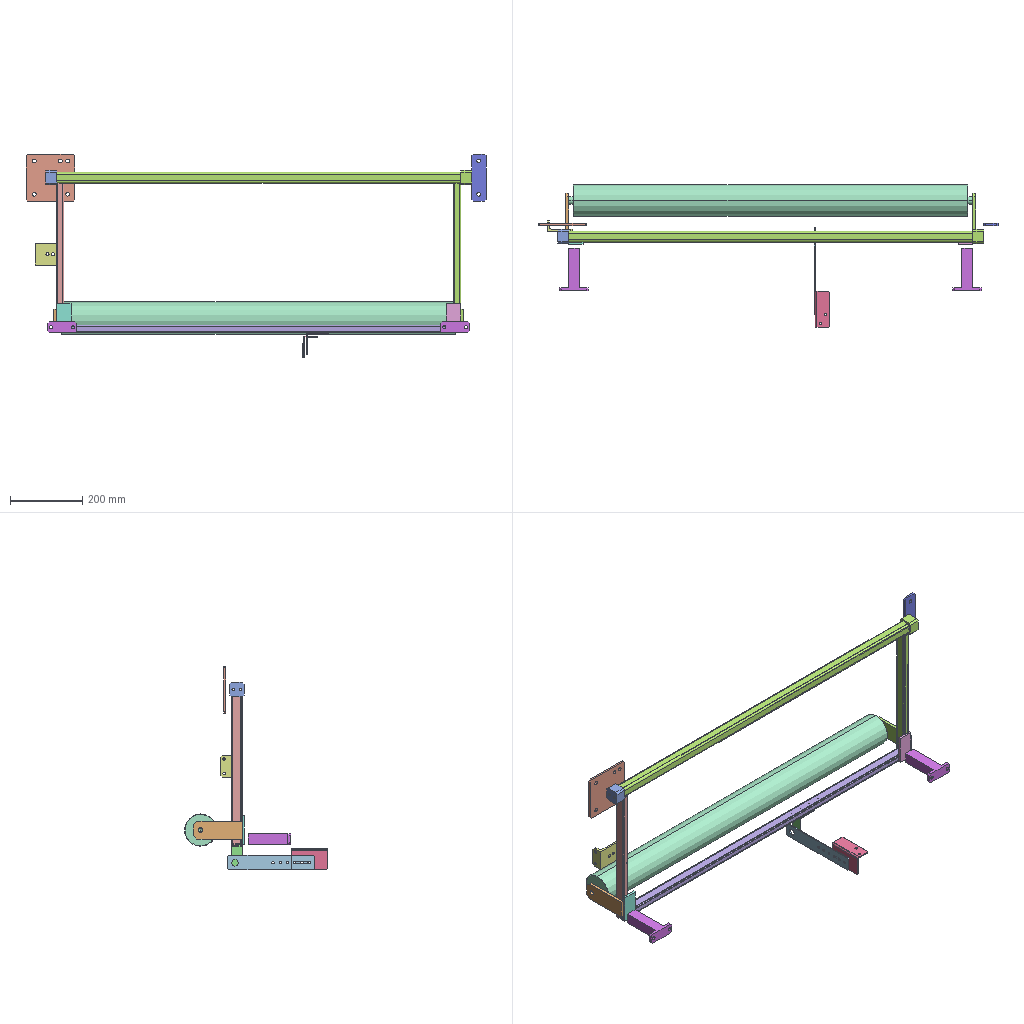Assembly | SolidWorks | 10 different items | 11 placed | box 1270 x 394 x 563 mm
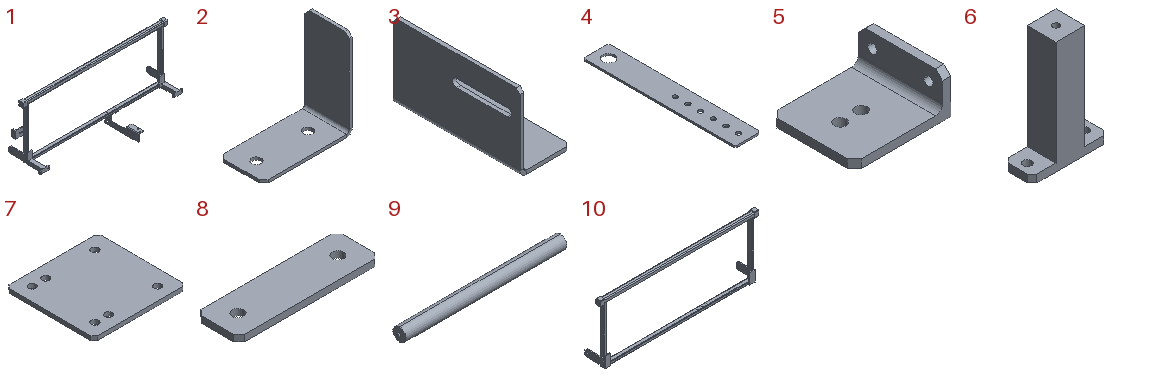Parts list (item | name | quantity | parent item | size | volume | features):
1 | (subassembly) | x1 | - | 1205 x 370 x 518 mm | 1223127 mm3 | -
2 | - | x1 | in 1 | 60 x 30 x 60 mm | 6834 mm3 | features Chamfer 1, EdgeFlange 1, FlatPattern 1, ICE 1, SMBaseFlange 1, SheetMetal 1
3 | - | x1 | in 1 | 40 x 100 x 60 mm | 27517 mm3 | features Chamfer 1, EdgeFlange 1, FlatPattern 1, ICE 1, SMBaseFlange 1, SheetMetal 1
4 | - | x1 | in 1 | 40 x 240 x 3 mm | 27247 mm3 | features Extrusion 1
5 | - | x1 | in 1 | 69 x 60 x 30 mm | 32423 mm3 | features ICE 3, Chamfer 1, Extrusion 1, Fillet 1
6 | - | x2 | in 1 | 80 x 30 x 118 mm | 115849 mm3 | features ICE 2, 3DProfileFeature 1, Extrusion 1, HoleWzd 1
7 | - | x1 | - | 135 x 130 x 6 mm | 101883 mm3 | features Extrusion 1
8 | - | x1 | - | 130 x 40 x 6 mm | 29861 mm3 | features Extrusion 1
9 | - | x1 | - | 1116 x 89 x 89 mm | 6785655 mm3 | features ICE 2, 3DProfileFeature 1, Extrusion 1, Fillet 1, HoleWzd 1
10 | - | x1 | in 1 | 1176 x 141 x 448 mm | 897407 mm3 | features ICE 5, 3DProfileFeature 4, HoleWzd 2, WeldMemberFeat 2, MirrorPattern 1, WeldmentFeature 1
Mates (type | each side: item.copy, entity, surface, feature):
In the top assembly
Concentric | 10.1 face cylinder Boss-Extrude3 | 9.1 face cylinder Boss-Extrude3
Coincident | 10.1 face plane Boss-Extrude3 | 9.1 face plane Boss-Extrude3
DistanceDim | 7.1 face plane Boss-Extrude1 | 10.1 face plane Boss-Extrude1
Width | 7.1 face plane Boss-Extrude1 | 7.1 face plane Boss-Extrude1 | 10.1 face plane Boss-Extrude1 | 10.1 face plane Boss-Extrude1
DistanceDim | 8.1 face plane Boss-Extrude1 | 10.1 face plane Mirror1
Width | 8.1 face plane Boss-Extrude1 | 8.1 face plane Boss-Extrude1 | 10.1 face plane Mirror1 | 10.1 face plane Mirror1
In subassembly 1
Coincident | 10.2 face plane Cold-formed hollow rectangular steel (GB/T 6728-2002) 30×20×2(1) | 2.1 face plane Base-Flange1
Concentric | 10.2 face cylinder M6 Tapped Hole1 | 2.1 face cylinder Cut-Extrude1 | 2 times
DistanceDim | 4.1 face plane Boss-Extrude1 | 2.1 face plane Edge-Flange1 | 2 times
DistanceDim | 2.1 face plane Edge-Flange1 | 4.1 face plane Boss-Extrude1
DistanceDim | 3.1 face plane Edge-Flange1 | 4.1 face plane Boss-Extrude1
Parallel | 3.1 face plane Edge-Flange1 | 4.1 face plane Boss-Extrude1
Concentric | 3.1 face cylinder Cut-Extrude1 | 4.1 face cylinder Boss-Extrude1
Coincident | 10.2 face plane Cold-formed hollow rectangular steel (GB/T 6728-2002) 30×20×2(1) | 5.1 face plane Boss-Extrude1
Width | 10.2 face plane Cold-formed hollow rectangular steel (GB/T 6728-2002) 30×20×2(1) | 10.2 face plane Cold-formed hollow square steel (GB/T 6728-2002) 30×3(1) | 5.1 face plane Boss-Extrude1 | 5.1 face plane Boss-Extrude1
DistanceDim | 5.1 face plane Boss-Extrude1 | 10.2 face plane Cold-formed hollow rectangular steel (GB/T 6728-2002) 30×20×2(1)
Coincident | 10.2 face plane Boss-Extrude2 | 6.1 face plane Boss-Extrude1
DistanceDim | 6.1 face plane Boss-Extrude2 | 10.2 face plane Boss-Extrude2
Coincident | 10.2 face plane Boss-Extrude2 | 6.1 face plane Boss-Extrude2
Coincident | 6.1 face plane Boss-Extrude1 | 6.2 face plane Boss-Extrude1
Coincident | 10.2 face plane Boss-Extrude2 | 6.2 face plane Boss-Extrude2
Coincident | 10.2 face plane Boss-Extrude2 | 6.2 face plane Boss-Extrude1